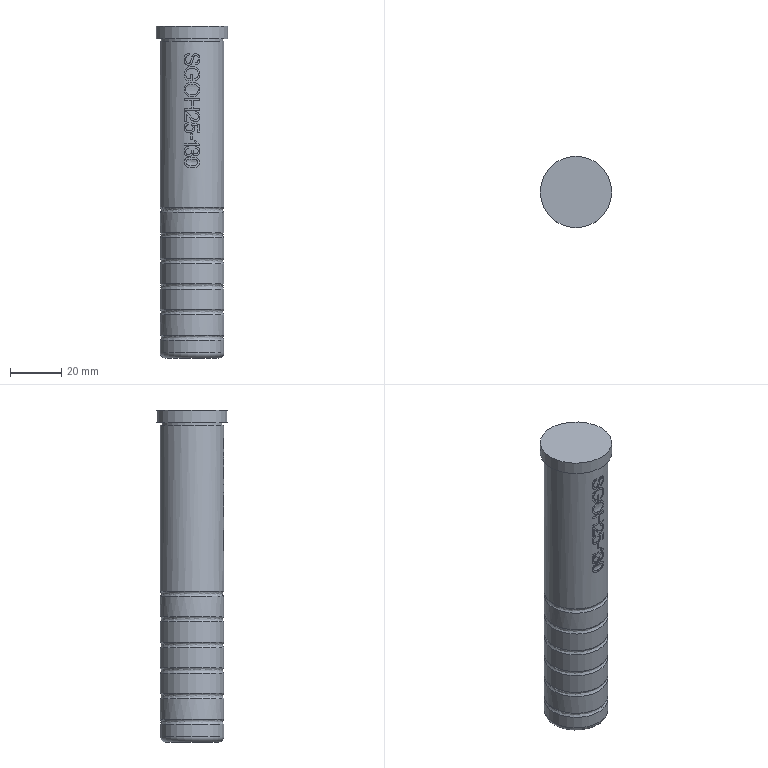Part | NX | features MI_SGOH_0850 2 | 1 solid | 164 faces | box 28 x 28 x 130 mm | volume 63999 mm3 | plane 82 | cylinder 75 | spline 6 | torus 1 | commonest cylinder face diameters 24.8 x10 25 x9 3.568 x2 1.688 x1 1.748 x1 2.096 x1